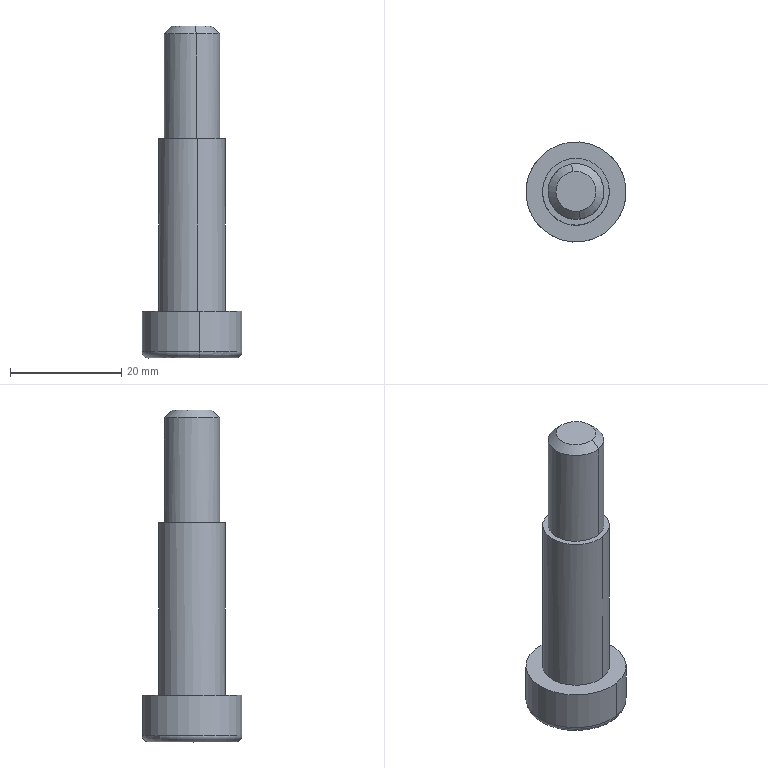Part | SolidWorks | features BaseBody 1 | 1 solid | 21 faces | box 18.001 x 18 x 59.642 mm | volume 7047 mm3 | plane 11 | cylinder 6 | torus 2 | cone 2 | commonest cylinder face diameters 10 x2 12 x2 18 x2